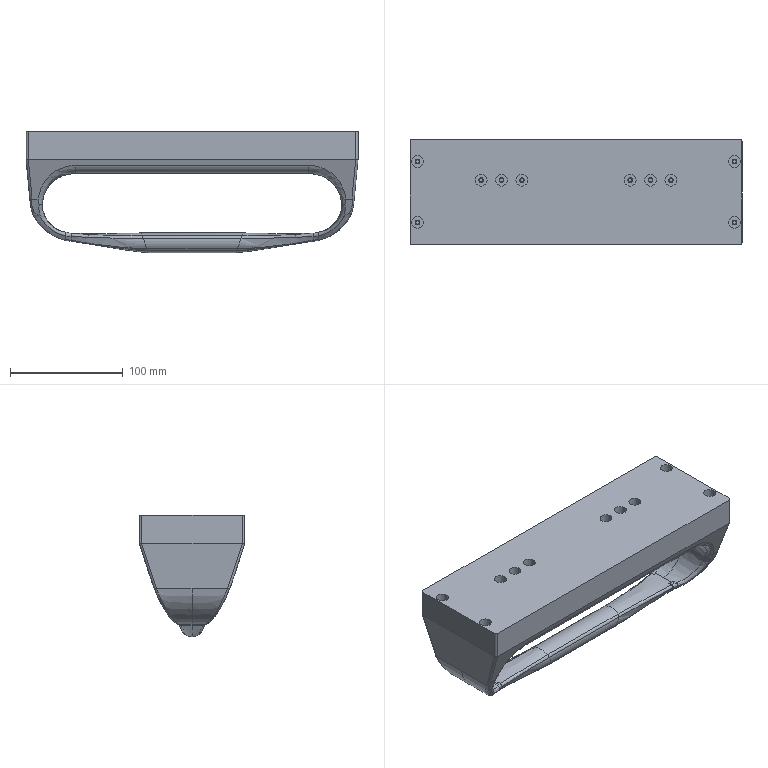Part | 2 solids | 250 faces | box 294.078 x 93.5 x 107.5 mm | volume 1064256 mm3 | cylinder 100 | plane 70 | spline 70 | cone 10 | commonest cylinder face diameters 6 x16 3.2 x10 4.2 x10 10.5 x10 12 x10 8 x4